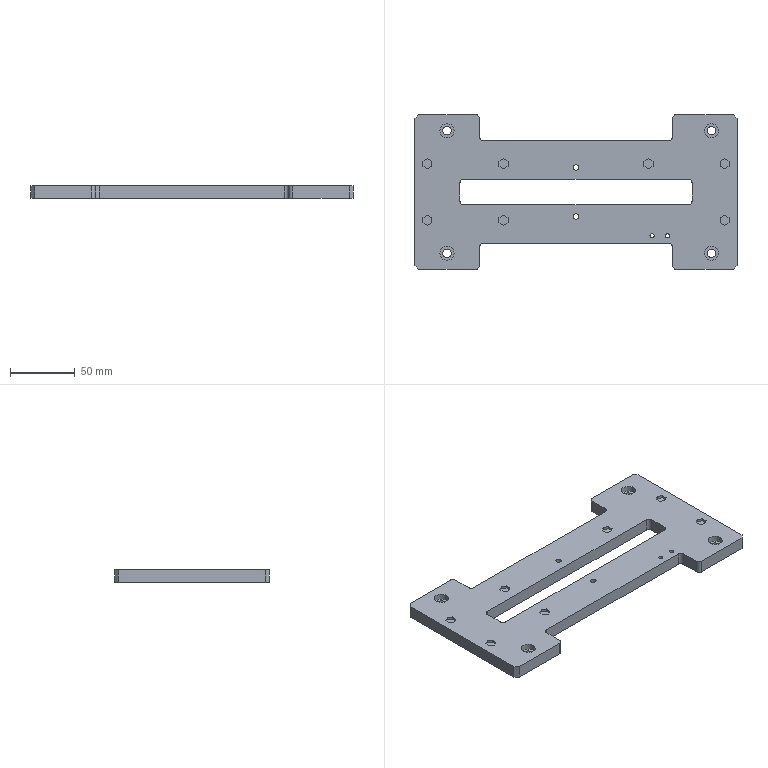Part | SolidWorks | features HoleWzd 3, Chamfer 1, Cut 1, Extrusion 1, Fillet 1 | 1 solid | 111 faces | box 250 x 120 x 10 mm | volume 200343 mm3 | plane 75 | cylinder 36 | commonest cylinder face diameters 6 x12 6.6 x8 11 x8 3.3 x4 4.2 x4